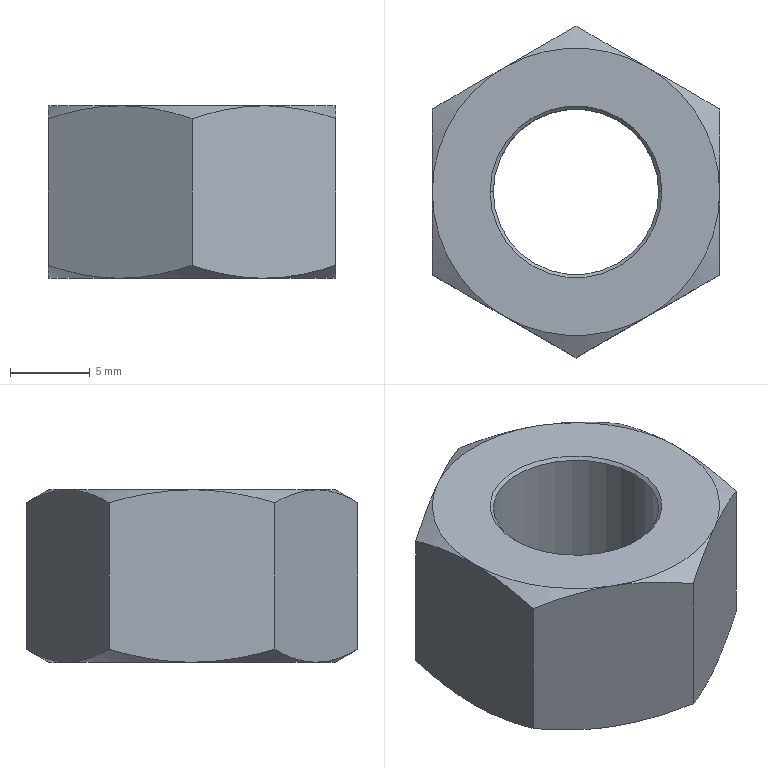Part | SolidWorks | features Cut 2, Chamfer 1, Extrusion 1 | 1 solid | 26 faces | box 18 x 20.785 x 10.8 mm | volume 2103 mm3 | cone 16 | plane 8 | cylinder 2 | commonest cylinder face diameters 10.376 x2
STEP:
#1=CARTESIAN_POINT('',(-5.188,0.,10.604));
#2=VERTEX_POINT('',#1);
#3=CARTESIAN_POINT('',(5.188,0.,10.604));
#4=VERTEX_POINT('',#3);
#5=CARTESIAN_POINT('',(0.,0.,10.604));
#6=DIRECTION('',(0.,0.,1.));
#7=DIRECTION('',(-1.,0.,0.));
#8=AXIS2_PLACEMENT_3D('',#5,#6,#7);
#9=CIRCLE('',#8,5.188);
#10=EDGE_CURVE('',#2,#4,#9,.T.);
#11=ORIENTED_EDGE('',*,*,#10,.F.);
#12=CARTESIAN_POINT('',(-5.385,0.,10.8));
#13=VERTEX_POINT('',#12);
#14=CARTESIAN_POINT('',(-5.188,0.,10.604));
#15=DIRECTION('',(-0.7071,0.,0.7071));
#16=VECTOR('',#15,1000.);
#17=LINE('',#14,#16);
#18=EDGE_CURVE('',#2,#13,#17,.T.);
#19=ORIENTED_EDGE('',*,*,#18,.T.);
#20=CARTESIAN_POINT('',(5.385,0.,10.8));
#21=VERTEX_POINT('',#20);
#22=CARTESIAN_POINT('',(0.,0.,10.8));
#23=DIRECTION('',(0.,0.,-1.));
#24=DIRECTION('',(-1.,0.,0.));
#25=AXIS2_PLACEMENT_3D('',#22,#23,#24);
#26=CIRCLE('',#25,5.385);
#27=EDGE_CURVE('',#21,#13,#26,.T.);
#28=ORIENTED_EDGE('',*,*,#27,.F.);
#29=CARTESIAN_POINT('',(5.188,0.,10.604));
#30=DIRECTION('',(0.7071,0.,0.7071));
#31=VECTOR('',#30,1000.);
#32=LINE('',#29,#31);
#33=EDGE_CURVE('',#4,#21,#32,.T.);
#34=ORIENTED_EDGE('',*,*,#33,.F.);
#35=EDGE_LOOP('',(#11,#19,#28,#34));
#36=FACE_OUTER_BOUND('',#35,.T.);
#37=CARTESIAN_POINT('',(0.,0.,10.604));
#38=DIRECTION('',(0.,0.,1.));
#39=DIRECTION('',(1.,0.,0.));
#40=AXIS2_PLACEMENT_3D('',#37,#38,#39);
#41=CONICAL_SURFACE('',#40,5.188,0.7854);
#42=ADVANCED_FACE('',(#36),#41,.F.);
#43=CARTESIAN_POINT('',(5.188,0.,0.1964));
#44=VERTEX_POINT('',#43);
#45=CARTESIAN_POINT('',(-5.188,0.,0.1964));
#46=VERTEX_POINT('',#45);
#47=CARTESIAN_POINT('',(0.,0.,0.1964));
#48=DIRECTION('',(0.,0.,-1.));
#49=DIRECTION('',(-1.,0.,0.));
#50=AXIS2_PLACEMENT_3D('',#47,#48,#49);
#51=CIRCLE('',#50,5.188);
#52=EDGE_CURVE('',#44,#46,#51,.T.);
#53=ORIENTED_EDGE('',*,*,#52,.F.);
#54=CARTESIAN_POINT('',(5.385,0.,0.));
#55=VERTEX_POINT('',#54);
#56=CARTESIAN_POINT('',(5.385,0.,0.));
#57=DIRECTION('',(0.7071,0.,-0.7071));
#58=VECTOR('',#57,1000.);
#59=LINE('',#56,#58);
#60=EDGE_CURVE('',#44,#55,#59,.T.);
#61=ORIENTED_EDGE('',*,*,#60,.T.);
#62=CARTESIAN_POINT('',(-5.385,0.,0.));
#63=VERTEX_POINT('',#62);
#64=CARTESIAN_POINT('',(0.,0.,0.));
#65=DIRECTION('',(0.,0.,1.));
#66=DIRECTION('',(-1.,0.,0.));
#67=AXIS2_PLACEMENT_3D('',#64,#65,#66);
#68=CIRCLE('',#67,5.385);
#69=EDGE_CURVE('',#63,#55,#68,.T.);
#70=ORIENTED_EDGE('',*,*,#69,.F.);
#71=CARTESIAN_POINT('',(-5.385,0.,0.));
#72=DIRECTION('',(-0.7071,0.,-0.7071));
#73=VECTOR('',#72,1000.);
#74=LINE('',#71,#73);
#75=EDGE_CURVE('',#46,#63,#74,.T.);
#76=ORIENTED_EDGE('',*,*,#75,.F.);
#77=EDGE_LOOP('',(#53,#61,#70,#76));
#78=FACE_OUTER_BOUND('',#77,.T.);
#79=CARTESIAN_POINT('',(0.,0.,0.));
#80=DIRECTION('',(0.,0.,-1.));
#81=DIRECTION('',(-1.,0.,0.));
#82=AXIS2_PLACEMENT_3D('',#79,#80,#81);
#83=CONICAL_SURFACE('',#82,5.385,0.7854);
#84=ADVANCED_FACE('',(#78),#83,.F.);
#85=ORIENTED_EDGE('',*,*,#10,.T.);
#86=CARTESIAN_POINT('',(5.188,0.,10.8));
#87=DIRECTION('',(0.,0.,-1.));
#88=VECTOR('',#87,1000.);
#89=LINE('',#86,#88);
#90=EDGE_CURVE('',#4,#44,#89,.T.);
#91=ORIENTED_EDGE('',*,*,#90,.T.);
#92=ORIENTED_EDGE('',*,*,#52,.T.);
#93=CARTESIAN_POINT('',(-5.188,0.,10.8));
#94=DIRECTION('',(0.,0.,-1.));
#95=VECTOR('',#94,1000.);
#96=LINE('',#93,#95);
#97=EDGE_CURVE('',#2,#46,#96,.T.);
#98=ORIENTED_EDGE('',*,*,#97,.F.);
#99=EDGE_LOOP('',(#85,#91,#92,#98));
#100=FACE_OUTER_BOUND('',#99,.T.);
#101=CARTESIAN_POINT('',(0.,0.,10.8));
#102=DIRECTION('',(0.,0.,-1.));
#103=DIRECTION('',(-1.,0.,0.));
#104=AXIS2_PLACEMENT_3D('',#101,#102,#103);
#105=CYLINDRICAL_SURFACE('',#104,5.188);
#106=ADVANCED_FACE('',(#100),#105,.F.);
#107=CARTESIAN_POINT('',(9.,5.196,9.996));
#108=VERTEX_POINT('',#107);
#109=CARTESIAN_POINT('',(4.5,7.794,10.8));
#110=VERTEX_POINT('',#109);
#111=CARTESIAN_POINT('',(9.,5.196,9.996));
#112=CARTESIAN_POINT('',(8.264,5.621,10.242));
#113=CARTESIAN_POINT('',(7.522,6.049,10.444));
#114=CARTESIAN_POINT('',(6.024,6.914,10.723));
#115=CARTESIAN_POINT('',(5.267,7.352,10.8));
#116=CARTESIAN_POINT('',(4.5,7.794,10.8));
#117=B_SPLINE_CURVE_WITH_KNOTS('',3,(#111,#112,#113,#114,#115,#116),.UNSPECIFIED.,.F.,.F.,(4,2,4),(0.000000238,0.002629,0.005258),.UNSPECIFIED.);
#118=EDGE_CURVE('',#108,#110,#117,.T.);
#119=ORIENTED_EDGE('',*,*,#118,.F.);
#120=CARTESIAN_POINT('',(9.,5.196,0.8038));
#121=VERTEX_POINT('',#120);
#122=CARTESIAN_POINT('',(9.,5.196,10.8));
#123=DIRECTION('',(0.,0.,-1.));
#124=VECTOR('',#123,1000.);
#125=LINE('',#122,#124);
#126=EDGE_CURVE('',#108,#121,#125,.T.);
#127=ORIENTED_EDGE('',*,*,#126,.T.);
#128=CARTESIAN_POINT('',(4.5,7.794,0.));
#129=VERTEX_POINT('',#128);
#130=CARTESIAN_POINT('',(4.5,7.794,0.));
#131=CARTESIAN_POINT('',(4.882,7.574,0.));
#132=CARTESIAN_POINT('',(5.266,7.352,0.019));
#133=CARTESIAN_POINT('',(6.024,6.914,0.09253));
#134=CARTESIAN_POINT('',(6.401,6.697,0.147));
#135=CARTESIAN_POINT('',(7.525,6.048,0.357));
#136=CARTESIAN_POINT('',(8.266,5.62,0.5591));
#137=CARTESIAN_POINT('',(9.,5.196,0.8038));
#138=B_SPLINE_CURVE_WITH_KNOTS('',3,(#130,#131,#132,#133,#134,#135,#136,#137),.UNSPECIFIED.,.F.,.F.,(4,2,2,4),(0.005258,0.006567,0.007877,0.0105),.UNSPECIFIED.);
#139=EDGE_CURVE('',#129,#121,#138,.T.);
#140=ORIENTED_EDGE('',*,*,#139,.F.);
#141=CARTESIAN_POINT('',(0.,10.392,0.8038));
#142=VERTEX_POINT('',#141);
#143=CARTESIAN_POINT('',(0.,10.392,0.8038));
#144=CARTESIAN_POINT('',(0.7361,9.967,0.5585));
#145=CARTESIAN_POINT('',(1.478,9.539,0.3563));
#146=CARTESIAN_POINT('',(2.976,8.674,0.07661));
#147=CARTESIAN_POINT('',(3.733,8.237,0.));
#148=CARTESIAN_POINT('',(4.5,7.794,0.));
#149=B_SPLINE_CURVE_WITH_KNOTS('',3,(#143,#144,#145,#146,#147,#148),.UNSPECIFIED.,.F.,.F.,(4,2,4),(0.000000238,0.002629,0.005258),.UNSPECIFIED.);
#150=EDGE_CURVE('',#142,#129,#149,.T.);
#151=ORIENTED_EDGE('',*,*,#150,.F.);
#152=CARTESIAN_POINT('',(0.,10.392,9.996));
#153=VERTEX_POINT('',#152);
#154=CARTESIAN_POINT('',(0.,10.392,10.8));
#155=DIRECTION('',(0.,0.,-1.));
#156=VECTOR('',#155,1000.);
#157=LINE('',#154,#156);
#158=EDGE_CURVE('',#153,#142,#157,.T.);
#159=ORIENTED_EDGE('',*,*,#158,.F.);
#160=CARTESIAN_POINT('',(4.5,7.794,10.8));
#161=CARTESIAN_POINT('',(4.118,8.015,10.8));
#162=CARTESIAN_POINT('',(3.734,8.236,10.781));
#163=CARTESIAN_POINT('',(2.976,8.674,10.707));
#164=CARTESIAN_POINT('',(2.599,8.892,10.653));
#165=CARTESIAN_POINT('',(1.475,9.541,10.443));
#166=CARTESIAN_POINT('',(0.7343,9.968,10.241));
#167=CARTESIAN_POINT('',(0.,10.392,9.996));
#168=B_SPLINE_CURVE_WITH_KNOTS('',3,(#160,#161,#162,#163,#164,#165,#166,#167),.UNSPECIFIED.,.F.,.F.,(4,2,2,4),(0.005258,0.006567,0.007877,0.0105),.UNSPECIFIED.);
#169=EDGE_CURVE('',#110,#153,#168,.T.);
#170=ORIENTED_EDGE('',*,*,#169,.F.);
#171=EDGE_LOOP('',(#119,#127,#140,#151,#159,#170));
#172=FACE_OUTER_BOUND('',#171,.T.);
#173=CARTESIAN_POINT('',(9.,5.196,10.8));
#174=DIRECTION('',(-0.5,-0.866,0.));
#175=DIRECTION('',(0.866,-0.5,0.));
#176=AXIS2_PLACEMENT_3D('',#173,#174,#175);
#177=PLANE('',#176);
#178=ADVANCED_FACE('',(#172),#177,.F.);
#179=CARTESIAN_POINT('',(-4.5,7.794,10.8));
#180=VERTEX_POINT('',#179);
#181=CARTESIAN_POINT('',(0.,10.392,9.996));
#182=CARTESIAN_POINT('',(-0.7361,9.967,10.242));
#183=CARTESIAN_POINT('',(-1.478,9.539,10.444));
#184=CARTESIAN_POINT('',(-2.976,8.674,10.723));
#185=CARTESIAN_POINT('',(-3.733,8.237,10.8));
#186=CARTESIAN_POINT('',(-4.5,7.794,10.8));
#187=B_SPLINE_CURVE_WITH_KNOTS('',3,(#181,#182,#183,#184,#185,#186),.UNSPECIFIED.,.F.,.F.,(4,2,4),(0.000000238,0.002629,0.005258),.UNSPECIFIED.);
#188=EDGE_CURVE('',#153,#180,#187,.T.);
#189=ORIENTED_EDGE('',*,*,#188,.F.);
#190=ORIENTED_EDGE('',*,*,#158,.T.);
#191=CARTESIAN_POINT('',(-4.5,7.794,0.));
#192=VERTEX_POINT('',#191);
#193=CARTESIAN_POINT('',(-4.5,7.794,0.));
#194=CARTESIAN_POINT('',(-4.118,8.015,0.));
#195=CARTESIAN_POINT('',(-3.734,8.236,0.019));
#196=CARTESIAN_POINT('',(-2.976,8.674,0.09253));
#197=CARTESIAN_POINT('',(-2.599,8.892,0.147));
#198=CARTESIAN_POINT('',(-1.475,9.541,0.357));
#199=CARTESIAN_POINT('',(-0.7343,9.968,0.5591));
#200=CARTESIAN_POINT('',(0.,10.392,0.8038));
#201=B_SPLINE_CURVE_WITH_KNOTS('',3,(#193,#194,#195,#196,#197,#198,#199,#200),.UNSPECIFIED.,.F.,.F.,(4,2,2,4),(0.005258,0.006567,0.007877,0.0105),.UNSPECIFIED.);
#202=EDGE_CURVE('',#192,#142,#201,.T.);
#203=ORIENTED_EDGE('',*,*,#202,.F.);
#204=CARTESIAN_POINT('',(-9.,5.196,0.8038));
#205=VERTEX_POINT('',#204);
#206=CARTESIAN_POINT('',(-9.,5.196,0.8038));
#207=CARTESIAN_POINT('',(-8.264,5.621,0.5585));
#208=CARTESIAN_POINT('',(-7.522,6.049,0.3563));
#209=CARTESIAN_POINT('',(-6.024,6.914,0.07661));
#210=CARTESIAN_POINT('',(-5.267,7.352,0.));
#211=CARTESIAN_POINT('',(-4.5,7.794,0.));
#212=B_SPLINE_CURVE_WITH_KNOTS('',3,(#206,#207,#208,#209,#210,#211),.UNSPECIFIED.,.F.,.F.,(4,2,4),(0.000000238,0.002629,0.005258),.UNSPECIFIED.);
#213=EDGE_CURVE('',#205,#192,#212,.T.);
#214=ORIENTED_EDGE('',*,*,#213,.F.);
#215=CARTESIAN_POINT('',(-9.,5.196,9.996));
#216=VERTEX_POINT('',#215);
#217=CARTESIAN_POINT('',(-9.,5.196,10.8));
#218=DIRECTION('',(0.,0.,-1.));
#219=VECTOR('',#218,1000.);
#220=LINE('',#217,#219);
#221=EDGE_CURVE('',#216,#205,#220,.T.);
#222=ORIENTED_EDGE('',*,*,#221,.F.);
#223=CARTESIAN_POINT('',(-4.5,7.794,10.8));
#224=CARTESIAN_POINT('',(-4.882,7.574,10.8));
#225=CARTESIAN_POINT('',(-5.266,7.352,10.781));
#226=CARTESIAN_POINT('',(-6.024,6.914,10.707));
#227=CARTESIAN_POINT('',(-6.401,6.697,10.653));
#228=CARTESIAN_POINT('',(-7.525,6.048,10.443));
#229=CARTESIAN_POINT('',(-8.266,5.62,10.241));
#230=CARTESIAN_POINT('',(-9.,5.196,9.996));
#231=B_SPLINE_CURVE_WITH_KNOTS('',3,(#223,#224,#225,#226,#227,#228,#229,#230),.UNSPECIFIED.,.F.,.F.,(4,2,2,4),(0.005258,0.006567,0.007877,0.0105),.UNSPECIFIED.);
#232=EDGE_CURVE('',#180,#216,#231,.T.);
#233=ORIENTED_EDGE('',*,*,#232,.F.);
#234=EDGE_LOOP('',(#189,#190,#203,#214,#222,#233));
#235=FACE_OUTER_BOUND('',#234,.T.);
#236=CARTESIAN_POINT('',(0.,10.392,10.8));
#237=DIRECTION('',(0.5,-0.866,0.));
#238=DIRECTION('',(0.866,0.5,0.));
#239=AXIS2_PLACEMENT_3D('',#236,#237,#238);
#240=PLANE('',#239);
#241=ADVANCED_FACE('',(#235),#240,.F.);
#242=CARTESIAN_POINT('',(-9.,0.,10.8));
#243=VERTEX_POINT('',#242);
#244=CARTESIAN_POINT('',(-9.,5.196,9.996));
#245=CARTESIAN_POINT('',(-9.,4.356,10.239));
#246=CARTESIAN_POINT('',(-9.,3.505,10.441));
#247=CARTESIAN_POINT('',(-9.,2.204,10.652));
#248=CARTESIAN_POINT('',(-9.,1.766,10.707));
#249=CARTESIAN_POINT('',(-9.,0.8814,10.781));
#250=CARTESIAN_POINT('',(-9.,0.4397,10.8));
#251=CARTESIAN_POINT('',(-9.,0.,10.8));
#252=B_SPLINE_CURVE_WITH_KNOTS('',3,(#244,#245,#246,#247,#248,#249,#250,#251),.UNSPECIFIED.,.F.,.F.,(4,2,2,4),(0.02958,0.03221,0.03352,0.03484),.UNSPECIFIED.);
#253=EDGE_CURVE('',#216,#243,#252,.T.);
#254=ORIENTED_EDGE('',*,*,#253,.F.);
#255=ORIENTED_EDGE('',*,*,#221,.T.);
#256=CARTESIAN_POINT('',(-9.,0.,0.));
#257=VERTEX_POINT('',#256);
#258=CARTESIAN_POINT('',(-9.,0.,0.));
#259=CARTESIAN_POINT('',(-9.,0.4397,0.));
#260=CARTESIAN_POINT('',(-9.,0.8814,0.01874));
#261=CARTESIAN_POINT('',(-9.,1.766,0.09308));
#262=CARTESIAN_POINT('',(-9.,2.204,0.1481));
#263=CARTESIAN_POINT('',(-9.,3.505,0.3593));
#264=CARTESIAN_POINT('',(-9.,4.356,0.5613));
#265=CARTESIAN_POINT('',(-9.,5.196,0.8038));
#266=B_SPLINE_CURVE_WITH_KNOTS('',3,(#258,#259,#260,#261,#262,#263,#264,#265),.UNSPECIFIED.,.F.,.F.,(4,2,2,4),(0.01478,0.01609,0.01741,0.02004),.UNSPECIFIED.);
#267=EDGE_CURVE('',#257,#205,#266,.T.);
#268=ORIENTED_EDGE('',*,*,#267,.F.);
#269=CARTESIAN_POINT('',(-9.,-5.196,0.8038));
#270=VERTEX_POINT('',#269);
#271=CARTESIAN_POINT('',(-9.,-5.196,0.8038));
#272=CARTESIAN_POINT('',(-9.,-4.35,0.5597));
#273=CARTESIAN_POINT('',(-9.,-3.485,0.3552));
#274=CARTESIAN_POINT('',(-9.,-1.751,0.07559));
#275=CARTESIAN_POINT('',(-9.,-0.8788,0.));
#276=CARTESIAN_POINT('',(-9.,0.,0.));
#277=B_SPLINE_CURVE_WITH_KNOTS('',3,(#271,#272,#273,#274,#275,#276),.UNSPECIFIED.,.F.,.F.,(4,2,4),(0.009518,0.01215,0.01478),.UNSPECIFIED.);
#278=EDGE_CURVE('',#270,#257,#277,.T.);
#279=ORIENTED_EDGE('',*,*,#278,.F.);
#280=CARTESIAN_POINT('',(-9.,-5.196,9.996));
#281=VERTEX_POINT('',#280);
#282=CARTESIAN_POINT('',(-9.,-5.196,10.8));
#283=DIRECTION('',(0.,0.,-1.));
#284=VECTOR('',#283,1000.);
#285=LINE('',#282,#284);
#286=EDGE_CURVE('',#281,#270,#285,.T.);
#287=ORIENTED_EDGE('',*,*,#286,.F.);
#288=CARTESIAN_POINT('',(-9.,0.,10.8));
#289=CARTESIAN_POINT('',(-9.,-0.8788,10.8));
#290=CARTESIAN_POINT('',(-9.,-1.751,10.724));
#291=CARTESIAN_POINT('',(-9.,-3.485,10.445));
#292=CARTESIAN_POINT('',(-9.,-4.35,10.24));
#293=CARTESIAN_POINT('',(-9.,-5.196,9.996));
#294=B_SPLINE_CURVE_WITH_KNOTS('',3,(#288,#289,#290,#291,#292,#293),.UNSPECIFIED.,.F.,.F.,(4,2,4),(0.03484,0.03747,0.0401),.UNSPECIFIED.);
#295=EDGE_CURVE('',#243,#281,#294,.T.);
#296=ORIENTED_EDGE('',*,*,#295,.F.);
#297=EDGE_LOOP('',(#254,#255,#268,#279,#287,#296));
#298=FACE_OUTER_BOUND('',#297,.T.);
#299=CARTESIAN_POINT('',(-9.,5.196,10.8));
#300=DIRECTION('',(1.,0.,0.));
#301=DIRECTION('',(0.,1.,0.));
#302=AXIS2_PLACEMENT_3D('',#299,#300,#301);
#303=PLANE('',#302);
#304=ADVANCED_FACE('',(#298),#303,.F.);
#305=CARTESIAN_POINT('',(-4.5,-7.794,10.8));
#306=VERTEX_POINT('',#305);
#307=CARTESIAN_POINT('',(-9.,-5.196,9.996));
#308=CARTESIAN_POINT('',(-8.264,-5.621,10.242));
#309=CARTESIAN_POINT('',(-7.522,-6.049,10.444));
#310=CARTESIAN_POINT('',(-6.024,-6.914,10.723));
#311=CARTESIAN_POINT('',(-5.267,-7.352,10.8));
#312=CARTESIAN_POINT('',(-4.5,-7.794,10.8));
#313=B_SPLINE_CURVE_WITH_KNOTS('',3,(#307,#308,#309,#310,#311,#312),.UNSPECIFIED.,.F.,.F.,(4,2,4),(0.000000238,0.002629,0.005258),.UNSPECIFIED.);
#314=EDGE_CURVE('',#281,#306,#313,.T.);
#315=ORIENTED_EDGE('',*,*,#314,.F.);
#316=ORIENTED_EDGE('',*,*,#286,.T.);
#317=CARTESIAN_POINT('',(-4.5,-7.794,0.));
#318=VERTEX_POINT('',#317);
#319=CARTESIAN_POINT('',(-4.5,-7.794,0.));
#320=CARTESIAN_POINT('',(-4.882,-7.574,0.));
#321=CARTESIAN_POINT('',(-5.266,-7.352,0.019));
#322=CARTESIAN_POINT('',(-6.024,-6.914,0.09253));
#323=CARTESIAN_POINT('',(-6.401,-6.697,0.147));
#324=CARTESIAN_POINT('',(-7.525,-6.048,0.357));
#325=CARTESIAN_POINT('',(-8.266,-5.62,0.5591));
#326=CARTESIAN_POINT('',(-9.,-5.196,0.8038));
#327=B_SPLINE_CURVE_WITH_KNOTS('',3,(#319,#320,#321,#322,#323,#324,#325,#326),.UNSPECIFIED.,.F.,.F.,(4,2,2,4),(0.005258,0.006567,0.007877,0.0105),.UNSPECIFIED.);
#328=EDGE_CURVE('',#318,#270,#327,.T.);
#329=ORIENTED_EDGE('',*,*,#328,.F.);
#330=CARTESIAN_POINT('',(0.,-10.392,0.8038));
#331=VERTEX_POINT('',#330);
#332=CARTESIAN_POINT('',(0.,-10.392,0.8038));
#333=CARTESIAN_POINT('',(-0.7361,-9.967,0.5585));
#334=CARTESIAN_POINT('',(-1.478,-9.539,0.3563));
#335=CARTESIAN_POINT('',(-2.976,-8.674,0.07661));
#336=CARTESIAN_POINT('',(-3.733,-8.237,0.));
#337=CARTESIAN_POINT('',(-4.5,-7.794,0.));
#338=B_SPLINE_CURVE_WITH_KNOTS('',3,(#332,#333,#334,#335,#336,#337),.UNSPECIFIED.,.F.,.F.,(4,2,4),(0.000000238,0.002629,0.005258),.UNSPECIFIED.);
#339=EDGE_CURVE('',#331,#318,#338,.T.);
#340=ORIENTED_EDGE('',*,*,#339,.F.);
#341=CARTESIAN_POINT('',(0.,-10.392,9.996));
#342=VERTEX_POINT('',#341);
#343=CARTESIAN_POINT('',(0.,-10.392,10.8));
#344=DIRECTION('',(0.,0.,-1.));
#345=VECTOR('',#344,1000.);
#346=LINE('',#343,#345);
#347=EDGE_CURVE('',#342,#331,#346,.T.);
#348=ORIENTED_EDGE('',*,*,#347,.F.);
#349=CARTESIAN_POINT('',(-4.5,-7.794,10.8));
#350=CARTESIAN_POINT('',(-4.118,-8.015,10.8));
#351=CARTESIAN_POINT('',(-3.734,-8.236,10.781));
#352=CARTESIAN_POINT('',(-2.976,-8.674,10.707));
#353=CARTESIAN_POINT('',(-2.599,-8.892,10.653));
#354=CARTESIAN_POINT('',(-1.475,-9.541,10.443));
#355=CARTESIAN_POINT('',(-0.7343,-9.968,10.241));
#356=CARTESIAN_POINT('',(0.,-10.392,9.996));
#357=B_SPLINE_CURVE_WITH_KNOTS('',3,(#349,#350,#351,#352,#353,#354,#355,#356),.UNSPECIFIED.,.F.,.F.,(4,2,2,4),(0.005258,0.006567,0.007877,0.0105),.UNSPECIFIED.);
#358=EDGE_CURVE('',#306,#342,#357,.T.);
#359=ORIENTED_EDGE('',*,*,#358,.F.);
#360=EDGE_LOOP('',(#315,#316,#329,#340,#348,#359));
#361=FACE_OUTER_BOUND('',#360,.T.);
#362=CARTESIAN_POINT('',(-9.,-5.196,10.8));
#363=DIRECTION('',(0.5,0.866,0.));
#364=DIRECTION('',(-0.866,0.5,0.));
#365=AXIS2_PLACEMENT_3D('',#362,#363,#364);
#366=PLANE('',#365);
#367=ADVANCED_FACE('',(#361),#366,.F.);
#368=CARTESIAN_POINT('',(4.5,-7.794,10.8));
#369=VERTEX_POINT('',#368);
#370=CARTESIAN_POINT('',(0.,-10.392,9.996));
#371=CARTESIAN_POINT('',(0.7361,-9.967,10.242));
#372=CARTESIAN_POINT('',(1.478,-9.539,10.444));
#373=CARTESIAN_POINT('',(2.976,-8.674,10.723));
#374=CARTESIAN_POINT('',(3.733,-8.237,10.8));
#375=CARTESIAN_POINT('',(4.5,-7.794,10.8));
#376=B_SPLINE_CURVE_WITH_KNOTS('',3,(#370,#371,#372,#373,#374,#375),.UNSPECIFIED.,.F.,.F.,(4,2,4),(0.000000238,0.002629,0.005258),.UNSPECIFIED.);
#377=EDGE_CURVE('',#342,#369,#376,.T.);
#378=ORIENTED_EDGE('',*,*,#377,.F.);
#379=ORIENTED_EDGE('',*,*,#347,.T.);
#380=CARTESIAN_POINT('',(4.5,-7.794,0.));
#381=VERTEX_POINT('',#380);
#382=CARTESIAN_POINT('',(4.5,-7.794,0.));
#383=CARTESIAN_POINT('',(4.118,-8.015,0.));
#384=CARTESIAN_POINT('',(3.734,-8.236,0.019));
#385=CARTESIAN_POINT('',(2.976,-8.674,0.09253));
#386=CARTESIAN_POINT('',(2.599,-8.892,0.147));
#387=CARTESIAN_POINT('',(1.475,-9.541,0.357));
#388=CARTESIAN_POINT('',(0.7343,-9.968,0.5591));
#389=CARTESIAN_POINT('',(0.,-10.392,0.8038));
#390=B_SPLINE_CURVE_WITH_KNOTS('',3,(#382,#383,#384,#385,#386,#387,#388,#389),.UNSPECIFIED.,.F.,.F.,(4,2,2,4),(0.005258,0.006567,0.007877,0.0105),.UNSPECIFIED.);
#391=EDGE_CURVE('',#381,#331,#390,.T.);
#392=ORIENTED_EDGE('',*,*,#391,.F.);
#393=CARTESIAN_POINT('',(9.,-5.196,0.8038));
#394=VERTEX_POINT('',#393);
#395=CARTESIAN_POINT('',(9.,-5.196,0.8038));
#396=CARTESIAN_POINT('',(8.264,-5.621,0.5585));
#397=CARTESIAN_POINT('',(7.522,-6.049,0.3563));
#398=CARTESIAN_POINT('',(6.024,-6.914,0.07661));
#399=CARTESIAN_POINT('',(5.267,-7.352,0.));
#400=CARTESIAN_POINT('',(4.5,-7.794,0.));
#401=B_SPLINE_CURVE_WITH_KNOTS('',3,(#395,#396,#397,#398,#399,#400),.UNSPECIFIED.,.F.,.F.,(4,2,4),(0.000000238,0.002629,0.005258),.UNSPECIFIED.);
#402=EDGE_CURVE('',#394,#381,#401,.T.);
#403=ORIENTED_EDGE('',*,*,#402,.F.);
#404=CARTESIAN_POINT('',(9.,-5.196,9.996));
#405=VERTEX_POINT('',#404);
#406=CARTESIAN_POINT('',(9.,-5.196,10.8));
#407=DIRECTION('',(0.,0.,-1.));
#408=VECTOR('',#407,1000.);
#409=LINE('',#406,#408);
#410=EDGE_CURVE('',#405,#394,#409,.T.);
#411=ORIENTED_EDGE('',*,*,#410,.F.);
#412=CARTESIAN_POINT('',(4.5,-7.794,10.8));
#413=CARTESIAN_POINT('',(4.882,-7.574,10.8));
#414=CARTESIAN_POINT('',(5.266,-7.352,10.781));
#415=CARTESIAN_POINT('',(6.024,-6.914,10.707));
#416=CARTESIAN_POINT('',(6.401,-6.697,10.653));
#417=CARTESIAN_POINT('',(7.525,-6.048,10.443));
#418=CARTESIAN_POINT('',(8.266,-5.62,10.241));
#419=CARTESIAN_POINT('',(9.,-5.196,9.996));
#420=B_SPLINE_CURVE_WITH_KNOTS('',3,(#412,#413,#414,#415,#416,#417,#418,#419),.UNSPECIFIED.,.F.,.F.,(4,2,2,4),(0.005258,0.006567,0.007877,0.0105),.UNSPECIFIED.);
#421=EDGE_CURVE('',#369,#405,#420,.T.);
#422=ORIENTED_EDGE('',*,*,#421,.F.);
#423=EDGE_LOOP('',(#378,#379,#392,#403,#411,#422));
#424=FACE_OUTER_BOUND('',#423,.T.);
#425=CARTESIAN_POINT('',(0.,-10.392,10.8));
#426=DIRECTION('',(-0.5,0.866,0.));
#427=DIRECTION('',(-0.866,-0.5,0.));
#428=AXIS2_PLACEMENT_3D('',#425,#426,#427);
#429=PLANE('',#428);
#430=ADVANCED_FACE('',(#424),#429,.F.);
#431=CARTESIAN_POINT('',(9.,0.,10.8));
#432=VERTEX_POINT('',#431);
#433=CARTESIAN_POINT('',(9.,-5.196,9.996));
#434=CARTESIAN_POINT('',(9.,-4.35,10.24));
#435=CARTESIAN_POINT('',(9.,-3.485,10.445));
#436=CARTESIAN_POINT('',(9.,-1.751,10.724));
#437=CARTESIAN_POINT('',(9.,-0.8788,10.8));
#438=CARTESIAN_POINT('',(9.,0.,10.8));
#439=B_SPLINE_CURVE_WITH_KNOTS('',3,(#433,#434,#435,#436,#437,#438),.UNSPECIFIED.,.F.,.F.,(4,2,4),(0.009518,0.01215,0.01478),.UNSPECIFIED.);
#440=EDGE_CURVE('',#405,#432,#439,.T.);
#441=ORIENTED_EDGE('',*,*,#440,.F.);
#442=ORIENTED_EDGE('',*,*,#410,.T.);
#443=CARTESIAN_POINT('',(9.,0.,0.));
#444=VERTEX_POINT('',#443);
#445=CARTESIAN_POINT('',(9.,0.,0.));
#446=CARTESIAN_POINT('',(9.,-0.8788,0.));
#447=CARTESIAN_POINT('',(9.,-1.751,0.07559));
#448=CARTESIAN_POINT('',(9.,-3.485,0.3552));
#449=CARTESIAN_POINT('',(9.,-4.35,0.5597));
#450=CARTESIAN_POINT('',(9.,-5.196,0.8038));
#451=B_SPLINE_CURVE_WITH_KNOTS('',3,(#445,#446,#447,#448,#449,#450),.UNSPECIFIED.,.F.,.F.,(4,2,4),(0.03484,0.03747,0.0401),.UNSPECIFIED.);
#452=EDGE_CURVE('',#444,#394,#451,.T.);
#453=ORIENTED_EDGE('',*,*,#452,.F.);
#454=CARTESIAN_POINT('',(9.,5.196,0.8038));
#455=CARTESIAN_POINT('',(9.,4.356,0.5613));
#456=CARTESIAN_POINT('',(9.,3.505,0.3593));
#457=CARTESIAN_POINT('',(9.,2.204,0.1481));
#458=CARTESIAN_POINT('',(9.,1.766,0.09308));
#459=CARTESIAN_POINT('',(9.,0.8814,0.01874));
#460=CARTESIAN_POINT('',(9.,0.4397,0.));
#461=CARTESIAN_POINT('',(9.,0.,0.));
#462=B_SPLINE_CURVE_WITH_KNOTS('',3,(#454,#455,#456,#457,#458,#459,#460,#461),.UNSPECIFIED.,.F.,.F.,(4,2,2,4),(0.02958,0.03221,0.03352,0.03484),.UNSPECIFIED.);
#463=EDGE_CURVE('',#121,#444,#462,.T.);
#464=ORIENTED_EDGE('',*,*,#463,.F.);
#465=ORIENTED_EDGE('',*,*,#126,.F.);
#466=CARTESIAN_POINT('',(9.,0.,10.8));
#467=CARTESIAN_POINT('',(9.,0.4397,10.8));
#468=CARTESIAN_POINT('',(9.,0.8814,10.781));
#469=CARTESIAN_POINT('',(9.,1.766,10.707));
#470=CARTESIAN_POINT('',(9.,2.204,10.652));
#471=CARTESIAN_POINT('',(9.,3.505,10.441));
#472=CARTESIAN_POINT('',(9.,4.356,10.239));
#473=CARTESIAN_POINT('',(9.,5.196,9.996));
#474=B_SPLINE_CURVE_WITH_KNOTS('',3,(#466,#467,#468,#469,#470,#471,#472,#473),.UNSPECIFIED.,.F.,.F.,(4,2,2,4),(0.01478,0.01609,0.01741,0.02004),.UNSPECIFIED.);
#475=EDGE_CURVE('',#432,#108,#474,.T.);
#476=ORIENTED_EDGE('',*,*,#475,.F.);
#477=EDGE_LOOP('',(#441,#442,#453,#464,#465,#476));
#478=FACE_OUTER_BOUND('',#477,.T.);
#479=CARTESIAN_POINT('',(9.,-5.196,10.8));
#480=DIRECTION('',(-1.,0.,0.));
#481=DIRECTION('',(0.,-1.,0.));
#482=AXIS2_PLACEMENT_3D('',#479,#480,#481);
#483=PLANE('',#482);
#484=ADVANCED_FACE('',(#478),#483,.F.);
#485=ORIENTED_EDGE('',*,*,#27,.T.);
#486=CARTESIAN_POINT('',(0.,0.,10.8));
#487=DIRECTION('',(0.,0.,-1.));
#488=DIRECTION('',(-1.,0.,0.));
#489=AXIS2_PLACEMENT_3D('',#486,#487,#488);
#490=CIRCLE('',#489,5.385);
#491=EDGE_CURVE('',#13,#21,#490,.T.);
#492=ORIENTED_EDGE('',*,*,#491,.T.);
#493=EDGE_LOOP('',(#485,#492));
#494=FACE_BOUND('',#493,.T.);
#495=CARTESIAN_POINT('',(0.,0.,10.8));
#496=DIRECTION('',(0.,0.,-1.));
#497=DIRECTION('',(-1.,0.,0.));
#498=AXIS2_PLACEMENT_3D('',#495,#496,#497);
#499=CIRCLE('',#498,9.);
#500=EDGE_CURVE('',#243,#180,#499,.T.);
#501=ORIENTED_EDGE('',*,*,#500,.F.);
#502=CARTESIAN_POINT('',(0.,0.,10.8));
#503=DIRECTION('',(0.,0.,-1.));
#504=DIRECTION('',(-1.,0.,0.));
#505=AXIS2_PLACEMENT_3D('',#502,#503,#504);
#506=CIRCLE('',#505,9.);
#507=EDGE_CURVE('',#306,#243,#506,.T.);
#508=ORIENTED_EDGE('',*,*,#507,.F.);
#509=CARTESIAN_POINT('',(0.,0.,10.8));
#510=DIRECTION('',(0.,0.,-1.));
#511=DIRECTION('',(-1.,0.,0.));
#512=AXIS2_PLACEMENT_3D('',#509,#510,#511);
#513=CIRCLE('',#512,9.);
#514=EDGE_CURVE('',#369,#306,#513,.T.);
#515=ORIENTED_EDGE('',*,*,#514,.F.);
#516=CARTESIAN_POINT('',(0.,0.,10.8));
#517=DIRECTION('',(0.,0.,-1.));
#518=DIRECTION('',(-1.,0.,0.));
#519=AXIS2_PLACEMENT_3D('',#516,#517,#518);
#520=CIRCLE('',#519,9.);
#521=EDGE_CURVE('',#432,#369,#520,.T.);
#522=ORIENTED_EDGE('',*,*,#521,.F.);
#523=CARTESIAN_POINT('',(0.,0.,10.8));
#524=DIRECTION('',(0.,0.,1.));
#525=DIRECTION('',(1.,0.,0.));
#526=AXIS2_PLACEMENT_3D('',#523,#524,#525);
#527=CIRCLE('',#526,9.);
#528=EDGE_CURVE('',#432,#110,#527,.T.);
#529=ORIENTED_EDGE('',*,*,#528,.T.);
#530=CARTESIAN_POINT('',(0.,0.,10.8));
#531=DIRECTION('',(0.,0.,-1.));
#532=DIRECTION('',(-1.,0.,0.));
#533=AXIS2_PLACEMENT_3D('',#530,#531,#532);
#534=CIRCLE('',#533,9.);
#535=EDGE_CURVE('',#180,#110,#534,.T.);
#536=ORIENTED_EDGE('',*,*,#535,.F.);
#537=EDGE_LOOP('',(#501,#508,#515,#522,#529,#536));
#538=FACE_OUTER_BOUND('',#537,.T.);
#539=CARTESIAN_POINT('',(9.,5.196,10.8));
#540=DIRECTION('',(0.,0.,-1.));
#541=DIRECTION('',(-1.,0.,0.));
#542=AXIS2_PLACEMENT_3D('',#539,#540,#541);
#543=PLANE('',#542);
#544=ADVANCED_FACE('',(#494,#538),#543,.F.);
#545=ORIENTED_EDGE('',*,*,#69,.T.);
#546=CARTESIAN_POINT('',(0.,0.,0.));
#547=DIRECTION('',(0.,0.,1.));
#548=DIRECTION('',(-1.,0.,0.));
#549=AXIS2_PLACEMENT_3D('',#546,#547,#548);
#550=CIRCLE('',#549,5.385);
#551=EDGE_CURVE('',#55,#63,#550,.T.);
#552=ORIENTED_EDGE('',*,*,#551,.T.);
#553=EDGE_LOOP('',(#545,#552));
#554=FACE_BOUND('',#553,.T.);
#555=CARTESIAN_POINT('',(0.,0.,0.));
#556=DIRECTION('',(0.,0.,-1.));
#557=DIRECTION('',(-1.,0.,0.));
#558=AXIS2_PLACEMENT_3D('',#555,#556,#557);
#559=CIRCLE('',#558,9.);
#560=EDGE_CURVE('',#318,#257,#559,.T.);
#561=ORIENTED_EDGE('',*,*,#560,.T.);
#562=CARTESIAN_POINT('',(0.,0.,0.));
#563=DIRECTION('',(0.,0.,-1.));
#564=DIRECTION('',(-1.,0.,0.));
#565=AXIS2_PLACEMENT_3D('',#562,#563,#564);
#566=CIRCLE('',#565,9.);
#567=EDGE_CURVE('',#257,#192,#566,.T.);
#568=ORIENTED_EDGE('',*,*,#567,.T.);
#569=CARTESIAN_POINT('',(0.,0.,0.));
#570=DIRECTION('',(0.,0.,-1.));
#571=DIRECTION('',(-1.,0.,0.));
#572=AXIS2_PLACEMENT_3D('',#569,#570,#571);
#573=CIRCLE('',#572,9.);
#574=EDGE_CURVE('',#192,#129,#573,.T.);
#575=ORIENTED_EDGE('',*,*,#574,.T.);
#576=CARTESIAN_POINT('',(0.,0.,0.));
#577=DIRECTION('',(0.,0.,-1.));
#578=DIRECTION('',(-1.,0.,0.));
#579=AXIS2_PLACEMENT_3D('',#576,#577,#578);
#580=CIRCLE('',#579,9.);
#581=EDGE_CURVE('',#129,#444,#580,.T.);
#582=ORIENTED_EDGE('',*,*,#581,.T.);
#583=CARTESIAN_POINT('',(0.,0.,0.));
#584=DIRECTION('',(0.,0.,-1.));
#585=DIRECTION('',(-1.,0.,0.));
#586=AXIS2_PLACEMENT_3D('',#583,#584,#585);
#587=CIRCLE('',#586,9.);
#588=EDGE_CURVE('',#444,#381,#587,.T.);
#589=ORIENTED_EDGE('',*,*,#588,.T.);
#590=CARTESIAN_POINT('',(0.,0.,0.));
#591=DIRECTION('',(0.,0.,-1.));
#592=DIRECTION('',(-1.,0.,0.));
#593=AXIS2_PLACEMENT_3D('',#590,#591,#592);
#594=CIRCLE('',#593,9.);
#595=EDGE_CURVE('',#381,#318,#594,.T.);
#596=ORIENTED_EDGE('',*,*,#595,.T.);
#597=EDGE_LOOP('',(#561,#568,#575,#582,#589,#596));
#598=FACE_OUTER_BOUND('',#597,.T.);
#599=CARTESIAN_POINT('',(9.,5.196,0.));
#600=DIRECTION('',(0.,0.,-1.));
#601=DIRECTION('',(-1.,0.,0.));
#602=AXIS2_PLACEMENT_3D('',#599,#600,#601);
#603=PLANE('',#602);
#604=ADVANCED_FACE('',(#554,#598),#603,.T.);
#605=ORIENTED_EDGE('',*,*,#90,.F.);
#606=CARTESIAN_POINT('',(0.,0.,10.604));
#607=DIRECTION('',(0.,0.,1.));
#608=DIRECTION('',(-1.,0.,0.));
#609=AXIS2_PLACEMENT_3D('',#606,#607,#608);
#610=CIRCLE('',#609,5.188);
#611=EDGE_CURVE('',#4,#2,#610,.T.);
#612=ORIENTED_EDGE('',*,*,#611,.T.);
#613=ORIENTED_EDGE('',*,*,#97,.T.);
#614=CARTESIAN_POINT('',(0.,0.,0.1964));
#615=DIRECTION('',(0.,0.,-1.));
#616=DIRECTION('',(-1.,0.,0.));
#617=AXIS2_PLACEMENT_3D('',#614,#615,#616);
#618=CIRCLE('',#617,5.188);
#619=EDGE_CURVE('',#46,#44,#618,.T.);
#620=ORIENTED_EDGE('',*,*,#619,.T.);
#621=EDGE_LOOP('',(#605,#612,#613,#620));
#622=FACE_OUTER_BOUND('',#621,.T.);
#623=CARTESIAN_POINT('',(0.,0.,10.8));
#624=DIRECTION('',(0.,0.,-1.));
#625=DIRECTION('',(-1.,0.,0.));
#626=AXIS2_PLACEMENT_3D('',#623,#624,#625);
#627=CYLINDRICAL_SURFACE('',#626,5.188);
#628=ADVANCED_FACE('',(#622),#627,.F.);
#629=ORIENTED_EDGE('',*,*,#402,.T.);
#630=ORIENTED_EDGE('',*,*,#588,.F.);
#631=ORIENTED_EDGE('',*,*,#452,.T.);
#632=EDGE_LOOP('',(#629,#630,#631));
#633=FACE_OUTER_BOUND('',#632,.T.);
#634=CARTESIAN_POINT('',(0.,0.,0.));
#635=DIRECTION('',(0.,0.,1.));
#636=DIRECTION('',(-1.,0.,0.));
#637=AXIS2_PLACEMENT_3D('',#634,#635,#636);
#638=CONICAL_SURFACE('',#637,9.,1.047);
#639=ADVANCED_FACE('',(#633),#638,.T.);
#640=ORIENTED_EDGE('',*,*,#139,.T.);
#641=ORIENTED_EDGE('',*,*,#463,.T.);
#642=ORIENTED_EDGE('',*,*,#581,.F.);
#643=EDGE_LOOP('',(#640,#641,#642));
#644=FACE_OUTER_BOUND('',#643,.T.);
#645=CARTESIAN_POINT('',(0.,0.,0.));
#646=DIRECTION('',(0.,0.,1.));
#647=DIRECTION('',(-1.,0.,0.));
#648=AXIS2_PLACEMENT_3D('',#645,#646,#647);
#649=CONICAL_SURFACE('',#648,9.,1.047);
#650=ADVANCED_FACE('',(#644),#649,.T.);
#651=ORIENTED_EDGE('',*,*,#339,.T.);
#652=ORIENTED_EDGE('',*,*,#595,.F.);
#653=ORIENTED_EDGE('',*,*,#391,.T.);
#654=EDGE_LOOP('',(#651,#652,#653));
#655=FACE_OUTER_BOUND('',#654,.T.);
#656=CARTESIAN_POINT('',(0.,0.,0.));
#657=DIRECTION('',(0.,0.,1.));
#658=DIRECTION('',(-1.,0.,0.));
#659=AXIS2_PLACEMENT_3D('',#656,#657,#658);
#660=CONICAL_SURFACE('',#659,9.,1.047);
#661=ADVANCED_FACE('',(#655),#660,.T.);
#662=ORIENTED_EDGE('',*,*,#278,.T.);
#663=ORIENTED_EDGE('',*,*,#560,.F.);
#664=ORIENTED_EDGE('',*,*,#328,.T.);
#665=EDGE_LOOP('',(#662,#663,#664));
#666=FACE_OUTER_BOUND('',#665,.T.);
#667=CARTESIAN_POINT('',(0.,0.,0.));
#668=DIRECTION('',(0.,0.,1.));
#669=DIRECTION('',(-1.,0.,0.));
#670=AXIS2_PLACEMENT_3D('',#667,#668,#669);
#671=CONICAL_SURFACE('',#670,9.,1.047);
#672=ADVANCED_FACE('',(#666),#671,.T.);
#673=ORIENTED_EDGE('',*,*,#267,.T.);
#674=ORIENTED_EDGE('',*,*,#213,.T.);
#675=ORIENTED_EDGE('',*,*,#567,.F.);
#676=EDGE_LOOP('',(#673,#674,#675));
#677=FACE_OUTER_BOUND('',#676,.T.);
#678=CARTESIAN_POINT('',(0.,0.,0.));
#679=DIRECTION('',(0.,0.,1.));
#680=DIRECTION('',(-1.,0.,0.));
#681=AXIS2_PLACEMENT_3D('',#678,#679,#680);
#682=CONICAL_SURFACE('',#681,9.,1.047);
#683=ADVANCED_FACE('',(#677),#682,.T.);
#684=ORIENTED_EDGE('',*,*,#202,.T.);
#685=ORIENTED_EDGE('',*,*,#150,.T.);
#686=ORIENTED_EDGE('',*,*,#574,.F.);
#687=EDGE_LOOP('',(#684,#685,#686));
#688=FACE_OUTER_BOUND('',#687,.T.);
#689=CARTESIAN_POINT('',(0.,0.,0.));
#690=DIRECTION('',(0.,0.,1.));
#691=DIRECTION('',(-1.,0.,0.));
#692=AXIS2_PLACEMENT_3D('',#689,#690,#691);
#693=CONICAL_SURFACE('',#692,9.,1.047);
#694=ADVANCED_FACE('',(#688),#693,.T.);
#695=ORIENTED_EDGE('',*,*,#295,.T.);
#696=ORIENTED_EDGE('',*,*,#314,.T.);
#697=ORIENTED_EDGE('',*,*,#507,.T.);
#698=EDGE_LOOP('',(#695,#696,#697));
#699=FACE_OUTER_BOUND('',#698,.T.);
#700=CARTESIAN_POINT('',(0.,0.,10.8));
#701=DIRECTION('',(0.,0.,-1.));
#702=DIRECTION('',(1.,0.,0.));
#703=AXIS2_PLACEMENT_3D('',#700,#701,#702);
#704=CONICAL_SURFACE('',#703,9.,1.047);
#705=ADVANCED_FACE('',(#699),#704,.T.);
#706=ORIENTED_EDGE('',*,*,#358,.T.);
#707=ORIENTED_EDGE('',*,*,#377,.T.);
#708=ORIENTED_EDGE('',*,*,#514,.T.);
#709=EDGE_LOOP('',(#706,#707,#708));
#710=FACE_OUTER_BOUND('',#709,.T.);
#711=CARTESIAN_POINT('',(0.,0.,10.8));
#712=DIRECTION('',(0.,0.,-1.));
#713=DIRECTION('',(1.,0.,0.));
#714=AXIS2_PLACEMENT_3D('',#711,#712,#713);
#715=CONICAL_SURFACE('',#714,9.,1.047);
#716=ADVANCED_FACE('',(#710),#715,.T.);
#717=ORIENTED_EDGE('',*,*,#421,.T.);
#718=ORIENTED_EDGE('',*,*,#440,.T.);
#719=ORIENTED_EDGE('',*,*,#521,.T.);
#720=EDGE_LOOP('',(#717,#718,#719));
#721=FACE_OUTER_BOUND('',#720,.T.);
#722=CARTESIAN_POINT('',(0.,0.,10.8));
#723=DIRECTION('',(0.,0.,-1.));
#724=DIRECTION('',(1.,0.,0.));
#725=AXIS2_PLACEMENT_3D('',#722,#723,#724);
#726=CONICAL_SURFACE('',#725,9.,1.047);
#727=ADVANCED_FACE('',(#721),#726,.T.);
#728=ORIENTED_EDGE('',*,*,#118,.T.);
#729=ORIENTED_EDGE('',*,*,#528,.F.);
#730=ORIENTED_EDGE('',*,*,#475,.T.);
#731=EDGE_LOOP('',(#728,#729,#730));
#732=FACE_OUTER_BOUND('',#731,.T.);
#733=CARTESIAN_POINT('',(0.,0.,10.8));
#734=DIRECTION('',(0.,0.,-1.));
#735=DIRECTION('',(1.,0.,0.));
#736=AXIS2_PLACEMENT_3D('',#733,#734,#735);
#737=CONICAL_SURFACE('',#736,9.,1.047);
#738=ADVANCED_FACE('',(#732),#737,.T.);
#739=ORIENTED_EDGE('',*,*,#169,.T.);
#740=ORIENTED_EDGE('',*,*,#188,.T.);
#741=ORIENTED_EDGE('',*,*,#535,.T.);
#742=EDGE_LOOP('',(#739,#740,#741));
#743=FACE_OUTER_BOUND('',#742,.T.);
#744=CARTESIAN_POINT('',(0.,0.,10.8));
#745=DIRECTION('',(0.,0.,-1.));
#746=DIRECTION('',(1.,0.,0.));
#747=AXIS2_PLACEMENT_3D('',#744,#745,#746);
#748=CONICAL_SURFACE('',#747,9.,1.047);
#749=ADVANCED_FACE('',(#743),#748,.T.);
#750=ORIENTED_EDGE('',*,*,#232,.T.);
#751=ORIENTED_EDGE('',*,*,#253,.T.);
#752=ORIENTED_EDGE('',*,*,#500,.T.);
#753=EDGE_LOOP('',(#750,#751,#752));
#754=FACE_OUTER_BOUND('',#753,.T.);
#755=CARTESIAN_POINT('',(0.,0.,10.8));
#756=DIRECTION('',(0.,0.,-1.));
#757=DIRECTION('',(1.,0.,0.));
#758=AXIS2_PLACEMENT_3D('',#755,#756,#757);
#759=CONICAL_SURFACE('',#758,9.,1.047);
#760=ADVANCED_FACE('',(#754),#759,.T.);
#761=ORIENTED_EDGE('',*,*,#60,.F.);
#762=ORIENTED_EDGE('',*,*,#619,.F.);
#763=ORIENTED_EDGE('',*,*,#75,.T.);
#764=ORIENTED_EDGE('',*,*,#551,.F.);
#765=EDGE_LOOP('',(#761,#762,#763,#764));
#766=FACE_OUTER_BOUND('',#765,.T.);
#767=CARTESIAN_POINT('',(0.,0.,0.));
#768=DIRECTION('',(0.,0.,-1.));
#769=DIRECTION('',(-1.,0.,0.));
#770=AXIS2_PLACEMENT_3D('',#767,#768,#769);
#771=CONICAL_SURFACE('',#770,5.385,0.7854);
#772=ADVANCED_FACE('',(#766),#771,.F.);
#773=ORIENTED_EDGE('',*,*,#18,.F.);
#774=ORIENTED_EDGE('',*,*,#611,.F.);
#775=ORIENTED_EDGE('',*,*,#33,.T.);
#776=ORIENTED_EDGE('',*,*,#491,.F.);
#777=EDGE_LOOP('',(#773,#774,#775,#776));
#778=FACE_OUTER_BOUND('',#777,.T.);
#779=CARTESIAN_POINT('',(0.,0.,10.604));
#780=DIRECTION('',(0.,0.,1.));
#781=DIRECTION('',(1.,0.,0.));
#782=AXIS2_PLACEMENT_3D('',#779,#780,#781);
#783=CONICAL_SURFACE('',#782,5.188,0.7854);
#784=ADVANCED_FACE('',(#778),#783,.F.);
#785=CLOSED_SHELL('',(#42,#84,#106,#178,#241,#304,#367,#430,#484,#544,#604,#628,#639,#650,#661,#672,#683,#694,#705,#716,#727,#738,#749,#760,#772,#784));
#786=MANIFOLD_SOLID_BREP('',#785);
#787=CARTESIAN_POINT('',(0.,0.,0.));
#788=DIRECTION('',(0.,0.,1.));
#789=DIRECTION('',(1.,0.,0.));
#790=AXIS2_PLACEMENT_3D('',#787,#788,#789);
#791=(LENGTH_UNIT()NAMED_UNIT(*)SI_UNIT(.MILLI.,.METRE.));
#792=UNCERTAINTY_MEASURE_WITH_UNIT(LENGTH_MEASURE(0.00001),#791,'','');
#793=(NAMED_UNIT(*)PLANE_ANGLE_UNIT()SI_UNIT($,.RADIAN.));
#794=(NAMED_UNIT(*)SI_UNIT($,.STERADIAN.)SOLID_ANGLE_UNIT());
#795=(GEOMETRIC_REPRESENTATION_CONTEXT(3)GLOBAL_UNCERTAINTY_ASSIGNED_CONTEXT((#792))GLOBAL_UNIT_ASSIGNED_CONTEXT((#791,#793,#794))REPRESENTATION_CONTEXT('',''));
#796=ADVANCED_BREP_SHAPE_REPRESENTATION('',(#786,#790),#795);